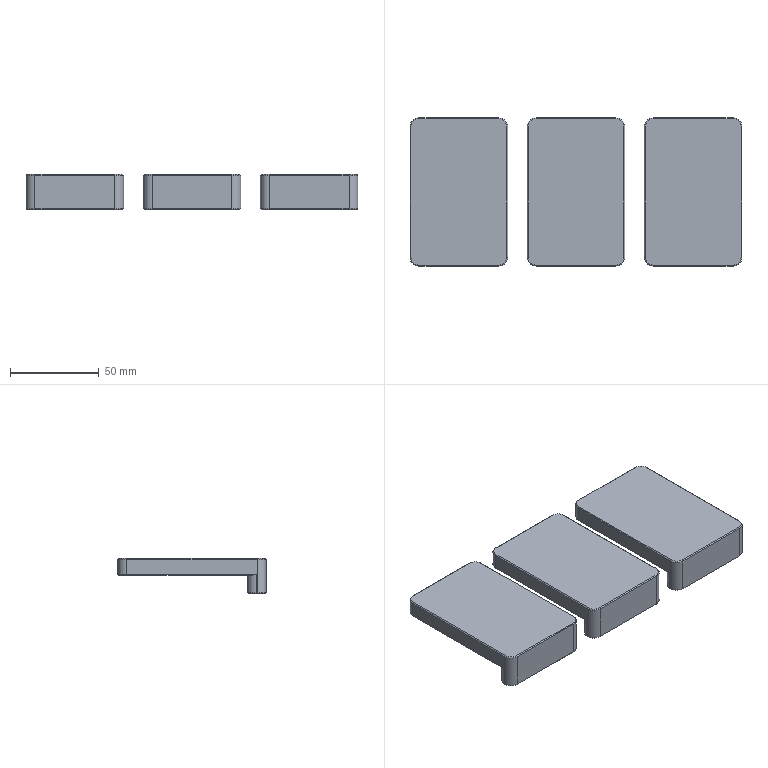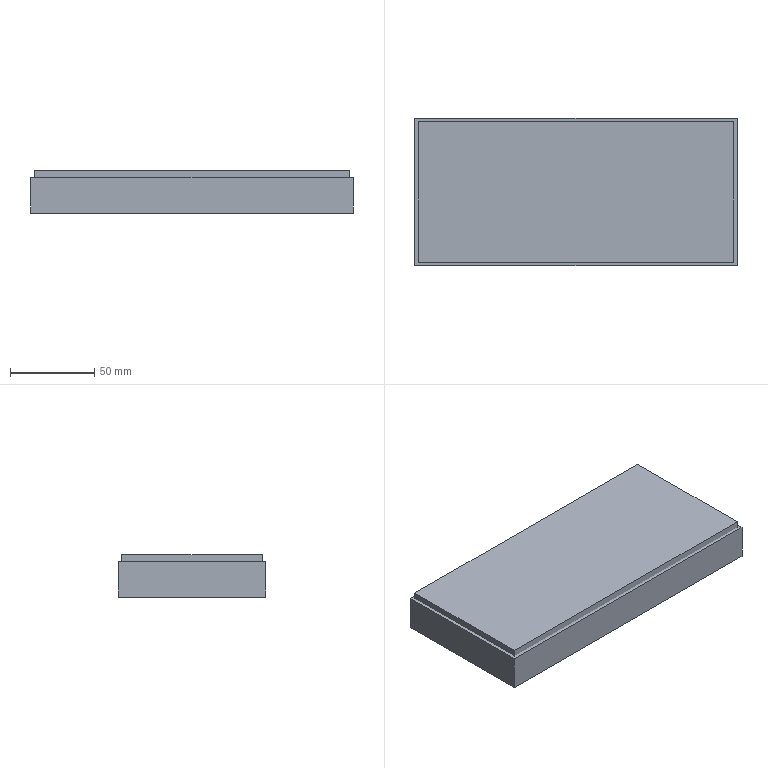CAM job | NX | 3-axis milling | part box 187 x 83.5 x 20 mm | stock box 191 x 87.5 x 25 mm
Tools:
number,name,description,diameter,corner_radius,flute_length,length,flutes
19,D80,Milling Tool-5 Parameters,80.0,0.0,50.0,75.0,2
15,D10,Milling Tool-5 Parameters,10.0,0.0,50.0,75.0,2
14,D10JING,Milling Tool-5 Parameters,10.0,0.0,50.0,75.0,2
1,D6A45,Milling Tool-5 Parameters,6.0,0.0,50.0,75.0,2
11,D4,Milling Tool-5 Parameters,4.0,0.0,50.0,75.0,2
Operations:
program,operation,operation_type,tool,method,geometry_group,spindle_rpm,surface_speed,feed_per_tooth,feed_cut,feed_plunge,cut_length_mm,path_length_mm,cut_time_min,machine_time_min
1,FLOOR_WALL,VolumeBased25DMillingOperation,D80,METHOD,A,6500.0,1633.0,0.1154,1500.0,100.0,609.497,663.497,0.4063,0.4117
1,ZLEVEL_PROFILE_COPY_1,ZLevelMilling,D10,METHOD,A,9500.0,298.0,0.1842,3500.0,1000.0,19076.122,19681.065,5.553,5.613
1,ZLEVEL_PROFILE_COPY_1_COPY,ZLevelMilling,D10JING,METHOD,A,9500.0,298.0,0.0632,1200.0,1000.0,2139.214,2740.306,1.988,2.048
1,PLANAR_MILL_COPY_COPY_COPY_COPY,PlanarMilling,D6A45,METHOD,A,9500.0,179.0,0.0658,1250.0,100.0,844.23,1215.679,0.6754,0.7125
2,FLOOR_WALL_COPY,VolumeBased25DMillingOperation,D80,METHOD,B,6500.0,1633.0,0.1154,1500.0,100.0,3007.485,3463.474,2.005,2.051
2,FLOOR_WALL_1,VolumeBased25DMillingOperation,D10,METHOD,B,9500.0,298.0,0.1316,2500.0,100.0,28308.718,28983.192,11.323,11.391
2,FLOOR_WALL_2,VolumeBased25DMillingOperation,D10JING,METHOD,B,9500.0,298.0,0.0789,1500.0,100.0,3294.338,4691.616,2.196,2.336
2,HOLE_MILLING,CylinderMilling,D4,METHOD,B,9500.0,119.0,0.0658,1250.0,100.0,2049.088,3405.103,1.639,1.775
2,PLANAR_MILL_COPY_COPY_COPY_COPY_COPY,PlanarMilling,D6A45,METHOD,B,9500.0,179.0,0.0658,1250.0,100.0,526.195,1243.433,0.421,0.4927
2,PLANAR_MILL_COPY_COPY_COPY_COPY_COPY_COPY,PlanarMilling,D6A45,METHOD,B,9500.0,179.0,0.0658,1250.0,100.0,748.386,2006.079,0.5987,0.7245
2,HOLE_MILLING_COPY,CylinderMilling,D4,METHOD,B,9500.0,119.0,0.0658,1250.0,100.0,518.884,1874.899,0.4151,0.5507